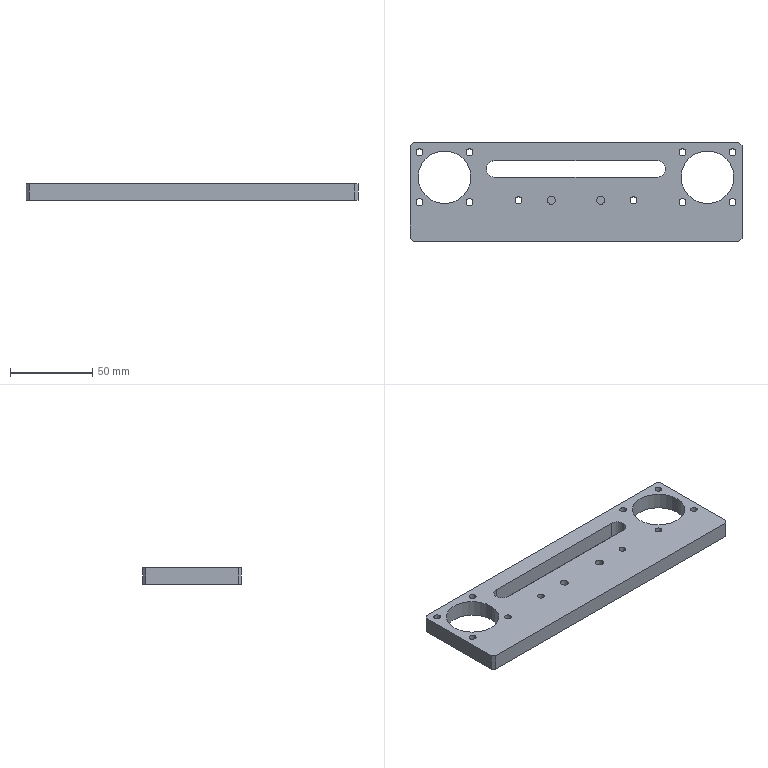Part | STEP file | 1 solid | 45 faces | box 202 x 60 x 10 mm | volume 92729 mm3 | cylinder 31 | plane 14 | commonest cylinder face diameters 4.2 x20 5 x4 32 x4 10 x3